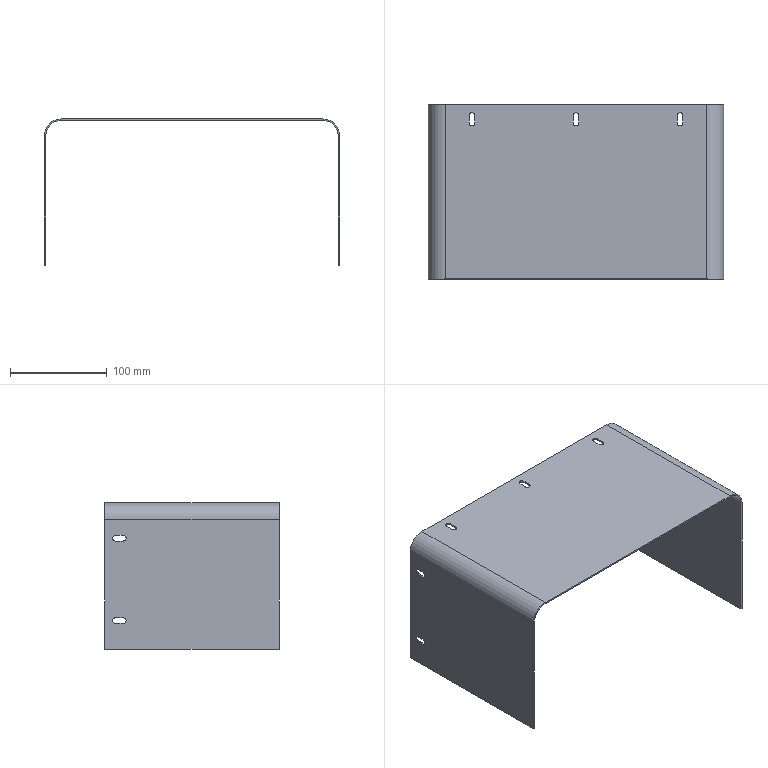Part | SolidWorks | features Fillet 2, HoleWzd 2, Shell 2, Extrusion 1, ICE 1 | 1 solid | 42 faces | box 305 x 180 x 151 mm | volume 158433 mm3 | plane 24 | cylinder 18 | commonest cylinder face diameters 5.8 x14 32 x2 35 x2
STEP:
#1=CARTESIAN_POINT('',(152.5,90.,58.));
#2=VERTEX_POINT('',#1);
#3=CARTESIAN_POINT('',(152.5,90.,-75.5));
#4=VERTEX_POINT('',#3);
#5=CARTESIAN_POINT('',(152.5,90.,75.5));
#6=DIRECTION('',(0.,0.,-1.));
#7=VECTOR('',#6,1000.);
#8=LINE('',#5,#7);
#9=EDGE_CURVE('',#2,#4,#8,.T.);
#10=ORIENTED_EDGE('',*,*,#9,.F.);
#11=CARTESIAN_POINT('',(152.5,-90.,58.));
#12=VERTEX_POINT('',#11);
#13=CARTESIAN_POINT('',(152.5,90.,58.));
#14=DIRECTION('',(0.,-1.,0.));
#15=VECTOR('',#14,1000.);
#16=LINE('',#13,#15);
#17=EDGE_CURVE('',#2,#12,#16,.T.);
#18=ORIENTED_EDGE('',*,*,#17,.T.);
#19=CARTESIAN_POINT('',(152.5,-90.,-75.5));
#20=VERTEX_POINT('',#19);
#21=CARTESIAN_POINT('',(152.5,-90.,75.5));
#22=DIRECTION('',(0.,0.,-1.));
#23=VECTOR('',#22,1000.);
#24=LINE('',#21,#23);
#25=EDGE_CURVE('',#12,#20,#24,.T.);
#26=ORIENTED_EDGE('',*,*,#25,.T.);
#27=CARTESIAN_POINT('',(152.5,90.,-75.5));
#28=DIRECTION('',(0.,-1.,0.));
#29=VECTOR('',#28,1000.);
#30=LINE('',#27,#29);
#31=EDGE_CURVE('',#4,#20,#30,.T.);
#32=ORIENTED_EDGE('',*,*,#31,.F.);
#33=EDGE_LOOP('',(#10,#18,#26,#32));
#34=FACE_OUTER_BOUND('',#33,.T.);
#35=CARTESIAN_POINT('',(152.5,71.,41.9));
#36=VERTEX_POINT('',#35);
#37=CARTESIAN_POINT('',(152.5,79.,41.9));
#38=VERTEX_POINT('',#37);
#39=CARTESIAN_POINT('',(152.5,71.,41.9));
#40=DIRECTION('',(0.,1.,0.));
#41=VECTOR('',#40,1000.);
#42=LINE('',#39,#41);
#43=EDGE_CURVE('',#36,#38,#42,.T.);
#44=ORIENTED_EDGE('',*,*,#43,.T.);
#45=CARTESIAN_POINT('',(152.5,79.,36.1));
#46=VERTEX_POINT('',#45);
#47=CARTESIAN_POINT('',(152.5,79.,39.));
#48=DIRECTION('',(-1.,0.,0.));
#49=DIRECTION('',(0.,0.,1.));
#50=AXIS2_PLACEMENT_3D('',#47,#48,#49);
#51=CIRCLE('',#50,2.9);
#52=EDGE_CURVE('',#38,#46,#51,.T.);
#53=ORIENTED_EDGE('',*,*,#52,.T.);
#54=CARTESIAN_POINT('',(152.5,71.,36.1));
#55=VERTEX_POINT('',#54);
#56=CARTESIAN_POINT('',(152.5,71.,36.1));
#57=DIRECTION('',(0.,1.,0.));
#58=VECTOR('',#57,1000.);
#59=LINE('',#56,#58);
#60=EDGE_CURVE('',#55,#46,#59,.T.);
#61=ORIENTED_EDGE('',*,*,#60,.F.);
#62=CARTESIAN_POINT('',(152.5,71.,39.));
#63=DIRECTION('',(-1.,0.,0.));
#64=DIRECTION('',(0.,0.,1.));
#65=AXIS2_PLACEMENT_3D('',#62,#63,#64);
#66=CIRCLE('',#65,2.9);
#67=EDGE_CURVE('',#55,#36,#66,.T.);
#68=ORIENTED_EDGE('',*,*,#67,.T.);
#69=EDGE_LOOP('',(#44,#53,#61,#68));
#70=FACE_BOUND('',#69,.T.);
#71=CARTESIAN_POINT('',(152.5,71.,-48.9));
#72=VERTEX_POINT('',#71);
#73=CARTESIAN_POINT('',(152.5,79.,-48.9));
#74=VERTEX_POINT('',#73);
#75=CARTESIAN_POINT('',(152.5,71.,-48.9));
#76=DIRECTION('',(0.,1.,0.));
#77=VECTOR('',#76,1000.);
#78=LINE('',#75,#77);
#79=EDGE_CURVE('',#72,#74,#78,.T.);
#80=ORIENTED_EDGE('',*,*,#79,.F.);
#81=CARTESIAN_POINT('',(152.5,71.,-43.1));
#82=VERTEX_POINT('',#81);
#83=CARTESIAN_POINT('',(152.5,71.,-46.));
#84=DIRECTION('',(-1.,0.,0.));
#85=DIRECTION('',(0.,0.,1.));
#86=AXIS2_PLACEMENT_3D('',#83,#84,#85);
#87=CIRCLE('',#86,2.9);
#88=EDGE_CURVE('',#72,#82,#87,.T.);
#89=ORIENTED_EDGE('',*,*,#88,.T.);
#90=CARTESIAN_POINT('',(152.5,79.,-43.1));
#91=VERTEX_POINT('',#90);
#92=CARTESIAN_POINT('',(152.5,71.,-43.1));
#93=DIRECTION('',(0.,1.,0.));
#94=VECTOR('',#93,1000.);
#95=LINE('',#92,#94);
#96=EDGE_CURVE('',#82,#91,#95,.T.);
#97=ORIENTED_EDGE('',*,*,#96,.T.);
#98=CARTESIAN_POINT('',(152.5,79.,-46.));
#99=DIRECTION('',(-1.,0.,0.));
#100=DIRECTION('',(0.,0.,1.));
#101=AXIS2_PLACEMENT_3D('',#98,#99,#100);
#102=CIRCLE('',#101,2.9);
#103=EDGE_CURVE('',#91,#74,#102,.T.);
#104=ORIENTED_EDGE('',*,*,#103,.T.);
#105=EDGE_LOOP('',(#80,#89,#97,#104));
#106=FACE_BOUND('',#105,.T.);
#107=CARTESIAN_POINT('',(152.5,90.,75.5));
#108=DIRECTION('',(-1.,0.,0.));
#109=DIRECTION('',(0.,0.,1.));
#110=AXIS2_PLACEMENT_3D('',#107,#108,#109);
#111=PLANE('',#110);
#112=ADVANCED_FACE('',(#34,#70,#106),#111,.F.);
#113=CARTESIAN_POINT('',(151.,90.,-75.5));
#114=VERTEX_POINT('',#113);
#115=CARTESIAN_POINT('',(151.,-90.,-75.5));
#116=VERTEX_POINT('',#115);
#117=CARTESIAN_POINT('',(151.,90.,-75.5));
#118=DIRECTION('',(0.,-1.,0.));
#119=VECTOR('',#118,1000.);
#120=LINE('',#117,#119);
#121=EDGE_CURVE('',#114,#116,#120,.T.);
#122=ORIENTED_EDGE('',*,*,#121,.F.);
#123=CARTESIAN_POINT('',(-152.5,90.,-75.5));
#124=DIRECTION('',(-1.,0.,0.));
#125=VECTOR('',#124,1000.);
#126=LINE('',#123,#125);
#127=EDGE_CURVE('',#4,#114,#126,.T.);
#128=ORIENTED_EDGE('',*,*,#127,.F.);
#129=ORIENTED_EDGE('',*,*,#31,.T.);
#130=CARTESIAN_POINT('',(-152.5,-90.,-75.5));
#131=DIRECTION('',(-1.,0.,0.));
#132=VECTOR('',#131,1000.);
#133=LINE('',#130,#132);
#134=EDGE_CURVE('',#20,#116,#133,.T.);
#135=ORIENTED_EDGE('',*,*,#134,.T.);
#136=EDGE_LOOP('',(#122,#128,#129,#135));
#137=FACE_OUTER_BOUND('',#136,.T.);
#138=CARTESIAN_POINT('',(-152.5,90.,-75.5));
#139=DIRECTION('',(0.,0.,1.));
#140=DIRECTION('',(1.,0.,0.));
#141=AXIS2_PLACEMENT_3D('',#138,#139,#140);
#142=PLANE('',#141);
#143=ADVANCED_FACE('',(#137),#142,.F.);
#144=CARTESIAN_POINT('',(151.,-90.,58.));
#145=VERTEX_POINT('',#144);
#146=CARTESIAN_POINT('',(135.,-90.,74.));
#147=VERTEX_POINT('',#146);
#148=CARTESIAN_POINT('',(135.,-90.,58.));
#149=DIRECTION('',(0.,-1.,0.));
#150=DIRECTION('',(0.,0.,-1.));
#151=AXIS2_PLACEMENT_3D('',#148,#149,#150);
#152=CIRCLE('',#151,16.);
#153=EDGE_CURVE('',#145,#147,#152,.T.);
#154=ORIENTED_EDGE('',*,*,#153,.F.);
#155=CARTESIAN_POINT('',(151.,-90.,0.));
#156=DIRECTION('',(0.,0.,-1.));
#157=VECTOR('',#156,1000.);
#158=LINE('',#155,#157);
#159=EDGE_CURVE('',#145,#116,#158,.T.);
#160=ORIENTED_EDGE('',*,*,#159,.T.);
#161=ORIENTED_EDGE('',*,*,#134,.F.);
#162=ORIENTED_EDGE('',*,*,#25,.F.);
#163=CARTESIAN_POINT('',(135.,-90.,75.5));
#164=VERTEX_POINT('',#163);
#165=CARTESIAN_POINT('',(135.,-90.,58.));
#166=DIRECTION('',(0.,-1.,0.));
#167=DIRECTION('',(0.,0.,-1.));
#168=AXIS2_PLACEMENT_3D('',#165,#166,#167);
#169=CIRCLE('',#168,17.5);
#170=EDGE_CURVE('',#12,#164,#169,.T.);
#171=ORIENTED_EDGE('',*,*,#170,.T.);
#172=CARTESIAN_POINT('',(-135.,-90.,75.5));
#173=VERTEX_POINT('',#172);
#174=CARTESIAN_POINT('',(-152.5,-90.,75.5));
#175=DIRECTION('',(1.,0.,0.));
#176=VECTOR('',#175,1000.);
#177=LINE('',#174,#176);
#178=EDGE_CURVE('',#173,#164,#177,.T.);
#179=ORIENTED_EDGE('',*,*,#178,.F.);
#180=CARTESIAN_POINT('',(-152.5,-90.,58.));
#181=VERTEX_POINT('',#180);
#182=CARTESIAN_POINT('',(-135.,-90.,58.));
#183=DIRECTION('',(0.,-1.,0.));
#184=DIRECTION('',(0.,0.,-1.));
#185=AXIS2_PLACEMENT_3D('',#182,#183,#184);
#186=CIRCLE('',#185,17.5);
#187=EDGE_CURVE('',#173,#181,#186,.T.);
#188=ORIENTED_EDGE('',*,*,#187,.T.);
#189=CARTESIAN_POINT('',(-152.5,-90.,-75.5));
#190=VERTEX_POINT('',#189);
#191=CARTESIAN_POINT('',(-152.5,-90.,75.5));
#192=DIRECTION('',(0.,0.,1.));
#193=VECTOR('',#192,1000.);
#194=LINE('',#191,#193);
#195=EDGE_CURVE('',#190,#181,#194,.T.);
#196=ORIENTED_EDGE('',*,*,#195,.F.);
#197=CARTESIAN_POINT('',(-151.,-90.,-75.5));
#198=VERTEX_POINT('',#197);
#199=CARTESIAN_POINT('',(-152.5,-90.,-75.5));
#200=DIRECTION('',(-1.,0.,0.));
#201=VECTOR('',#200,1000.);
#202=LINE('',#199,#201);
#203=EDGE_CURVE('',#198,#190,#202,.T.);
#204=ORIENTED_EDGE('',*,*,#203,.F.);
#205=CARTESIAN_POINT('',(-151.,-90.,58.));
#206=VERTEX_POINT('',#205);
#207=CARTESIAN_POINT('',(-151.,-90.,0.));
#208=DIRECTION('',(0.,0.,1.));
#209=VECTOR('',#208,1000.);
#210=LINE('',#207,#209);
#211=EDGE_CURVE('',#198,#206,#210,.T.);
#212=ORIENTED_EDGE('',*,*,#211,.T.);
#213=CARTESIAN_POINT('',(-135.,-90.,74.));
#214=VERTEX_POINT('',#213);
#215=CARTESIAN_POINT('',(-135.,-90.,58.));
#216=DIRECTION('',(0.,-1.,0.));
#217=DIRECTION('',(0.,0.,-1.));
#218=AXIS2_PLACEMENT_3D('',#215,#216,#217);
#219=CIRCLE('',#218,16.);
#220=EDGE_CURVE('',#214,#206,#219,.T.);
#221=ORIENTED_EDGE('',*,*,#220,.F.);
#222=CARTESIAN_POINT('',(0.,-90.,74.));
#223=DIRECTION('',(1.,0.,0.));
#224=VECTOR('',#223,1000.);
#225=LINE('',#222,#224);
#226=EDGE_CURVE('',#214,#147,#225,.T.);
#227=ORIENTED_EDGE('',*,*,#226,.T.);
#228=EDGE_LOOP('',(#154,#160,#161,#162,#171,#179,#188,#196,#204,#212,#221,#227));
#229=FACE_OUTER_BOUND('',#228,.T.);
#230=CARTESIAN_POINT('',(0.,-90.,0.));
#231=DIRECTION('',(0.,-1.,0.));
#232=DIRECTION('',(0.,0.,-1.));
#233=AXIS2_PLACEMENT_3D('',#230,#231,#232);
#234=PLANE('',#233);
#235=ADVANCED_FACE('',(#229),#234,.T.);
#236=CARTESIAN_POINT('',(-151.,90.,-75.5));
#237=VERTEX_POINT('',#236);
#238=CARTESIAN_POINT('',(-152.5,90.,-75.5));
#239=VERTEX_POINT('',#238);
#240=CARTESIAN_POINT('',(-152.5,90.,-75.5));
#241=DIRECTION('',(-1.,0.,0.));
#242=VECTOR('',#241,1000.);
#243=LINE('',#240,#242);
#244=EDGE_CURVE('',#237,#239,#243,.T.);
#245=ORIENTED_EDGE('',*,*,#244,.F.);
#246=CARTESIAN_POINT('',(-151.,90.,-75.5));
#247=DIRECTION('',(0.,-1.,0.));
#248=VECTOR('',#247,1000.);
#249=LINE('',#246,#248);
#250=EDGE_CURVE('',#237,#198,#249,.T.);
#251=ORIENTED_EDGE('',*,*,#250,.T.);
#252=ORIENTED_EDGE('',*,*,#203,.T.);
#253=CARTESIAN_POINT('',(-152.5,90.,-75.5));
#254=DIRECTION('',(0.,-1.,0.));
#255=VECTOR('',#254,1000.);
#256=LINE('',#253,#255);
#257=EDGE_CURVE('',#239,#190,#256,.T.);
#258=ORIENTED_EDGE('',*,*,#257,.F.);
#259=EDGE_LOOP('',(#245,#251,#252,#258));
#260=FACE_OUTER_BOUND('',#259,.T.);
#261=CARTESIAN_POINT('',(-152.5,90.,-75.5));
#262=DIRECTION('',(0.,0.,1.));
#263=DIRECTION('',(1.,0.,0.));
#264=AXIS2_PLACEMENT_3D('',#261,#262,#263);
#265=PLANE('',#264);
#266=ADVANCED_FACE('',(#260),#265,.F.);
#267=CARTESIAN_POINT('',(-152.5,71.,-48.9));
#268=VERTEX_POINT('',#267);
#269=CARTESIAN_POINT('',(-152.5,71.,-43.1));
#270=VERTEX_POINT('',#269);
#271=CARTESIAN_POINT('',(-152.5,71.,-46.));
#272=DIRECTION('',(-1.,0.,0.));
#273=DIRECTION('',(0.,0.,1.));
#274=AXIS2_PLACEMENT_3D('',#271,#272,#273);
#275=CIRCLE('',#274,2.9);
#276=EDGE_CURVE('',#268,#270,#275,.T.);
#277=ORIENTED_EDGE('',*,*,#276,.F.);
#278=CARTESIAN_POINT('',(-152.5,79.,-48.9));
#279=VERTEX_POINT('',#278);
#280=CARTESIAN_POINT('',(-152.5,71.,-48.9));
#281=DIRECTION('',(0.,1.,0.));
#282=VECTOR('',#281,1000.);
#283=LINE('',#280,#282);
#284=EDGE_CURVE('',#268,#279,#283,.T.);
#285=ORIENTED_EDGE('',*,*,#284,.T.);
#286=CARTESIAN_POINT('',(-152.5,79.,-43.1));
#287=VERTEX_POINT('',#286);
#288=CARTESIAN_POINT('',(-152.5,79.,-46.));
#289=DIRECTION('',(-1.,0.,0.));
#290=DIRECTION('',(0.,0.,1.));
#291=AXIS2_PLACEMENT_3D('',#288,#289,#290);
#292=CIRCLE('',#291,2.9);
#293=EDGE_CURVE('',#287,#279,#292,.T.);
#294=ORIENTED_EDGE('',*,*,#293,.F.);
#295=CARTESIAN_POINT('',(-152.5,71.,-43.1));
#296=DIRECTION('',(0.,1.,0.));
#297=VECTOR('',#296,1000.);
#298=LINE('',#295,#297);
#299=EDGE_CURVE('',#270,#287,#298,.T.);
#300=ORIENTED_EDGE('',*,*,#299,.F.);
#301=EDGE_LOOP('',(#277,#285,#294,#300));
#302=FACE_BOUND('',#301,.T.);
#303=CARTESIAN_POINT('',(-152.5,71.,36.1));
#304=VERTEX_POINT('',#303);
#305=CARTESIAN_POINT('',(-152.5,71.,41.9));
#306=VERTEX_POINT('',#305);
#307=CARTESIAN_POINT('',(-152.5,71.,39.));
#308=DIRECTION('',(-1.,0.,0.));
#309=DIRECTION('',(0.,0.,1.));
#310=AXIS2_PLACEMENT_3D('',#307,#308,#309);
#311=CIRCLE('',#310,2.9);
#312=EDGE_CURVE('',#304,#306,#311,.T.);
#313=ORIENTED_EDGE('',*,*,#312,.F.);
#314=CARTESIAN_POINT('',(-152.5,79.,36.1));
#315=VERTEX_POINT('',#314);
#316=CARTESIAN_POINT('',(-152.5,71.,36.1));
#317=DIRECTION('',(0.,1.,0.));
#318=VECTOR('',#317,1000.);
#319=LINE('',#316,#318);
#320=EDGE_CURVE('',#304,#315,#319,.T.);
#321=ORIENTED_EDGE('',*,*,#320,.T.);
#322=CARTESIAN_POINT('',(-152.5,79.,41.9));
#323=VERTEX_POINT('',#322);
#324=CARTESIAN_POINT('',(-152.5,79.,39.));
#325=DIRECTION('',(-1.,0.,0.));
#326=DIRECTION('',(0.,0.,1.));
#327=AXIS2_PLACEMENT_3D('',#324,#325,#326);
#328=CIRCLE('',#327,2.9);
#329=EDGE_CURVE('',#323,#315,#328,.T.);
#330=ORIENTED_EDGE('',*,*,#329,.F.);
#331=CARTESIAN_POINT('',(-152.5,71.,41.9));
#332=DIRECTION('',(0.,1.,0.));
#333=VECTOR('',#332,1000.);
#334=LINE('',#331,#333);
#335=EDGE_CURVE('',#306,#323,#334,.T.);
#336=ORIENTED_EDGE('',*,*,#335,.F.);
#337=EDGE_LOOP('',(#313,#321,#330,#336));
#338=FACE_BOUND('',#337,.T.);
#339=ORIENTED_EDGE('',*,*,#195,.T.);
#340=CARTESIAN_POINT('',(-152.5,90.,58.));
#341=VERTEX_POINT('',#340);
#342=CARTESIAN_POINT('',(-152.5,90.,58.));
#343=DIRECTION('',(0.,1.,0.));
#344=VECTOR('',#343,1000.);
#345=LINE('',#342,#344);
#346=EDGE_CURVE('',#181,#341,#345,.T.);
#347=ORIENTED_EDGE('',*,*,#346,.T.);
#348=CARTESIAN_POINT('',(-152.5,90.,75.5));
#349=DIRECTION('',(0.,0.,1.));
#350=VECTOR('',#349,1000.);
#351=LINE('',#348,#350);
#352=EDGE_CURVE('',#239,#341,#351,.T.);
#353=ORIENTED_EDGE('',*,*,#352,.F.);
#354=ORIENTED_EDGE('',*,*,#257,.T.);
#355=EDGE_LOOP('',(#339,#347,#353,#354));
#356=FACE_OUTER_BOUND('',#355,.T.);
#357=CARTESIAN_POINT('',(-152.5,90.,75.5));
#358=DIRECTION('',(1.,0.,0.));
#359=DIRECTION('',(0.,0.,-1.));
#360=AXIS2_PLACEMENT_3D('',#357,#358,#359);
#361=PLANE('',#360);
#362=ADVANCED_FACE('',(#302,#338,#356),#361,.F.);
#363=CARTESIAN_POINT('',(-110.4,71.,75.5));
#364=VERTEX_POINT('',#363);
#365=CARTESIAN_POINT('',(-104.6,71.,75.5));
#366=VERTEX_POINT('',#365);
#367=CARTESIAN_POINT('',(-107.5,71.,75.5));
#368=DIRECTION('',(0.,0.,1.));
#369=DIRECTION('',(1.,0.,0.));
#370=AXIS2_PLACEMENT_3D('',#367,#368,#369);
#371=CIRCLE('',#370,2.9);
#372=EDGE_CURVE('',#364,#366,#371,.T.);
#373=ORIENTED_EDGE('',*,*,#372,.F.);
#374=CARTESIAN_POINT('',(-110.4,79.,75.5));
#375=VERTEX_POINT('',#374);
#376=CARTESIAN_POINT('',(-110.4,71.,75.5));
#377=DIRECTION('',(0.,1.,0.));
#378=VECTOR('',#377,1000.);
#379=LINE('',#376,#378);
#380=EDGE_CURVE('',#364,#375,#379,.T.);
#381=ORIENTED_EDGE('',*,*,#380,.T.);
#382=CARTESIAN_POINT('',(-104.6,79.,75.5));
#383=VERTEX_POINT('',#382);
#384=CARTESIAN_POINT('',(-107.5,79.,75.5));
#385=DIRECTION('',(0.,0.,1.));
#386=DIRECTION('',(1.,0.,0.));
#387=AXIS2_PLACEMENT_3D('',#384,#385,#386);
#388=CIRCLE('',#387,2.9);
#389=EDGE_CURVE('',#383,#375,#388,.T.);
#390=ORIENTED_EDGE('',*,*,#389,.F.);
#391=CARTESIAN_POINT('',(-104.6,71.,75.5));
#392=DIRECTION('',(0.,1.,0.));
#393=VECTOR('',#392,1000.);
#394=LINE('',#391,#393);
#395=EDGE_CURVE('',#366,#383,#394,.T.);
#396=ORIENTED_EDGE('',*,*,#395,.F.);
#397=EDGE_LOOP('',(#373,#381,#390,#396));
#398=FACE_BOUND('',#397,.T.);
#399=CARTESIAN_POINT('',(-2.9,71.,75.5));
#400=VERTEX_POINT('',#399);
#401=CARTESIAN_POINT('',(2.9,71.,75.5));
#402=VERTEX_POINT('',#401);
#403=CARTESIAN_POINT('',(0.,71.,75.5));
#404=DIRECTION('',(0.,0.,1.));
#405=DIRECTION('',(1.,0.,0.));
#406=AXIS2_PLACEMENT_3D('',#403,#404,#405);
#407=CIRCLE('',#406,2.9);
#408=EDGE_CURVE('',#400,#402,#407,.T.);
#409=ORIENTED_EDGE('',*,*,#408,.F.);
#410=CARTESIAN_POINT('',(-2.9,79.,75.5));
#411=VERTEX_POINT('',#410);
#412=CARTESIAN_POINT('',(-2.9,71.,75.5));
#413=DIRECTION('',(0.,1.,0.));
#414=VECTOR('',#413,1000.);
#415=LINE('',#412,#414);
#416=EDGE_CURVE('',#400,#411,#415,.T.);
#417=ORIENTED_EDGE('',*,*,#416,.T.);
#418=CARTESIAN_POINT('',(2.9,79.,75.5));
#419=VERTEX_POINT('',#418);
#420=CARTESIAN_POINT('',(0.,79.,75.5));
#421=DIRECTION('',(0.,0.,1.));
#422=DIRECTION('',(1.,0.,0.));
#423=AXIS2_PLACEMENT_3D('',#420,#421,#422);
#424=CIRCLE('',#423,2.9);
#425=EDGE_CURVE('',#419,#411,#424,.T.);
#426=ORIENTED_EDGE('',*,*,#425,.F.);
#427=CARTESIAN_POINT('',(2.9,71.,75.5));
#428=DIRECTION('',(0.,1.,0.));
#429=VECTOR('',#428,1000.);
#430=LINE('',#427,#429);
#431=EDGE_CURVE('',#402,#419,#430,.T.);
#432=ORIENTED_EDGE('',*,*,#431,.F.);
#433=EDGE_LOOP('',(#409,#417,#426,#432));
#434=FACE_BOUND('',#433,.T.);
#435=CARTESIAN_POINT('',(104.6,71.,75.5));
#436=VERTEX_POINT('',#435);
#437=CARTESIAN_POINT('',(110.4,71.,75.5));
#438=VERTEX_POINT('',#437);
#439=CARTESIAN_POINT('',(107.5,71.,75.5));
#440=DIRECTION('',(0.,0.,1.));
#441=DIRECTION('',(1.,0.,0.));
#442=AXIS2_PLACEMENT_3D('',#439,#440,#441);
#443=CIRCLE('',#442,2.9);
#444=EDGE_CURVE('',#436,#438,#443,.T.);
#445=ORIENTED_EDGE('',*,*,#444,.F.);
#446=CARTESIAN_POINT('',(104.6,79.,75.5));
#447=VERTEX_POINT('',#446);
#448=CARTESIAN_POINT('',(104.6,71.,75.5));
#449=DIRECTION('',(0.,1.,0.));
#450=VECTOR('',#449,1000.);
#451=LINE('',#448,#450);
#452=EDGE_CURVE('',#436,#447,#451,.T.);
#453=ORIENTED_EDGE('',*,*,#452,.T.);
#454=CARTESIAN_POINT('',(110.4,79.,75.5));
#455=VERTEX_POINT('',#454);
#456=CARTESIAN_POINT('',(107.5,79.,75.5));
#457=DIRECTION('',(0.,0.,1.));
#458=DIRECTION('',(1.,0.,0.));
#459=AXIS2_PLACEMENT_3D('',#456,#457,#458);
#460=CIRCLE('',#459,2.9);
#461=EDGE_CURVE('',#455,#447,#460,.T.);
#462=ORIENTED_EDGE('',*,*,#461,.F.);
#463=CARTESIAN_POINT('',(110.4,71.,75.5));
#464=DIRECTION('',(0.,1.,0.));
#465=VECTOR('',#464,1000.);
#466=LINE('',#463,#465);
#467=EDGE_CURVE('',#438,#455,#466,.T.);
#468=ORIENTED_EDGE('',*,*,#467,.F.);
#469=EDGE_LOOP('',(#445,#453,#462,#468));
#470=FACE_BOUND('',#469,.T.);
#471=ORIENTED_EDGE('',*,*,#178,.T.);
#472=CARTESIAN_POINT('',(135.,90.,75.5));
#473=VERTEX_POINT('',#472);
#474=CARTESIAN_POINT('',(135.,90.,75.5));
#475=DIRECTION('',(0.,1.,0.));
#476=VECTOR('',#475,1000.);
#477=LINE('',#474,#476);
#478=EDGE_CURVE('',#164,#473,#477,.T.);
#479=ORIENTED_EDGE('',*,*,#478,.T.);
#480=CARTESIAN_POINT('',(-135.,90.,75.5));
#481=VERTEX_POINT('',#480);
#482=CARTESIAN_POINT('',(-152.5,90.,75.5));
#483=DIRECTION('',(1.,0.,0.));
#484=VECTOR('',#483,1000.);
#485=LINE('',#482,#484);
#486=EDGE_CURVE('',#481,#473,#485,.T.);
#487=ORIENTED_EDGE('',*,*,#486,.F.);
#488=CARTESIAN_POINT('',(-135.,90.,75.5));
#489=DIRECTION('',(0.,-1.,0.));
#490=VECTOR('',#489,1000.);
#491=LINE('',#488,#490);
#492=EDGE_CURVE('',#481,#173,#491,.T.);
#493=ORIENTED_EDGE('',*,*,#492,.T.);
#494=EDGE_LOOP('',(#471,#479,#487,#493));
#495=FACE_OUTER_BOUND('',#494,.T.);
#496=CARTESIAN_POINT('',(-152.5,90.,75.5));
#497=DIRECTION('',(0.,0.,-1.));
#498=DIRECTION('',(-1.,0.,0.));
#499=AXIS2_PLACEMENT_3D('',#496,#497,#498);
#500=PLANE('',#499);
#501=ADVANCED_FACE('',(#398,#434,#470,#495),#500,.F.);
#502=CARTESIAN_POINT('',(151.,90.,58.));
#503=VERTEX_POINT('',#502);
#504=CARTESIAN_POINT('',(151.,90.,0.));
#505=DIRECTION('',(0.,0.,-1.));
#506=VECTOR('',#505,1000.);
#507=LINE('',#504,#506);
#508=EDGE_CURVE('',#503,#114,#507,.T.);
#509=ORIENTED_EDGE('',*,*,#508,.F.);
#510=CARTESIAN_POINT('',(135.,90.,74.));
#511=VERTEX_POINT('',#510);
#512=CARTESIAN_POINT('',(135.,90.,58.));
#513=DIRECTION('',(0.,1.,0.));
#514=DIRECTION('',(0.,0.,-1.));
#515=AXIS2_PLACEMENT_3D('',#512,#513,#514);
#516=CIRCLE('',#515,16.);
#517=EDGE_CURVE('',#511,#503,#516,.T.);
#518=ORIENTED_EDGE('',*,*,#517,.F.);
#519=CARTESIAN_POINT('',(-135.,90.,74.));
#520=VERTEX_POINT('',#519);
#521=CARTESIAN_POINT('',(0.,90.,74.));
#522=DIRECTION('',(1.,0.,0.));
#523=VECTOR('',#522,1000.);
#524=LINE('',#521,#523);
#525=EDGE_CURVE('',#520,#511,#524,.T.);
#526=ORIENTED_EDGE('',*,*,#525,.F.);
#527=CARTESIAN_POINT('',(-151.,90.,58.));
#528=VERTEX_POINT('',#527);
#529=CARTESIAN_POINT('',(-135.,90.,58.));
#530=DIRECTION('',(0.,1.,0.));
#531=DIRECTION('',(0.,0.,-1.));
#532=AXIS2_PLACEMENT_3D('',#529,#530,#531);
#533=CIRCLE('',#532,16.);
#534=EDGE_CURVE('',#528,#520,#533,.T.);
#535=ORIENTED_EDGE('',*,*,#534,.F.);
#536=CARTESIAN_POINT('',(-151.,90.,0.));
#537=DIRECTION('',(0.,0.,1.));
#538=VECTOR('',#537,1000.);
#539=LINE('',#536,#538);
#540=EDGE_CURVE('',#237,#528,#539,.T.);
#541=ORIENTED_EDGE('',*,*,#540,.F.);
#542=ORIENTED_EDGE('',*,*,#244,.T.);
#543=ORIENTED_EDGE('',*,*,#352,.T.);
#544=CARTESIAN_POINT('',(-135.,90.,58.));
#545=DIRECTION('',(0.,1.,0.));
#546=DIRECTION('',(0.,0.,-1.));
#547=AXIS2_PLACEMENT_3D('',#544,#545,#546);
#548=CIRCLE('',#547,17.5);
#549=EDGE_CURVE('',#341,#481,#548,.T.);
#550=ORIENTED_EDGE('',*,*,#549,.T.);
#551=ORIENTED_EDGE('',*,*,#486,.T.);
#552=CARTESIAN_POINT('',(135.,90.,58.));
#553=DIRECTION('',(0.,1.,0.));
#554=DIRECTION('',(0.,0.,-1.));
#555=AXIS2_PLACEMENT_3D('',#552,#553,#554);
#556=CIRCLE('',#555,17.5);
#557=EDGE_CURVE('',#473,#2,#556,.T.);
#558=ORIENTED_EDGE('',*,*,#557,.T.);
#559=ORIENTED_EDGE('',*,*,#9,.T.);
#560=ORIENTED_EDGE('',*,*,#127,.T.);
#561=EDGE_LOOP('',(#509,#518,#526,#535,#541,#542,#543,#550,#551,#558,#559,#560));
#562=FACE_OUTER_BOUND('',#561,.T.);
#563=CARTESIAN_POINT('',(0.,90.,0.));
#564=DIRECTION('',(0.,-1.,0.));
#565=DIRECTION('',(0.,0.,-1.));
#566=AXIS2_PLACEMENT_3D('',#563,#564,#565);
#567=PLANE('',#566);
#568=ADVANCED_FACE('',(#562),#567,.F.);
#569=ORIENTED_EDGE('',*,*,#557,.F.);
#570=ORIENTED_EDGE('',*,*,#478,.F.);
#571=ORIENTED_EDGE('',*,*,#170,.F.);
#572=ORIENTED_EDGE('',*,*,#17,.F.);
#573=EDGE_LOOP('',(#569,#570,#571,#572));
#574=FACE_OUTER_BOUND('',#573,.T.);
#575=CARTESIAN_POINT('',(135.,90.,58.));
#576=DIRECTION('',(0.,-1.,0.));
#577=DIRECTION('',(0.,0.,-1.));
#578=AXIS2_PLACEMENT_3D('',#575,#576,#577);
#579=CYLINDRICAL_SURFACE('',#578,17.5);
#580=ADVANCED_FACE('',(#574),#579,.T.);
#581=ORIENTED_EDGE('',*,*,#549,.F.);
#582=ORIENTED_EDGE('',*,*,#346,.F.);
#583=ORIENTED_EDGE('',*,*,#187,.F.);
#584=ORIENTED_EDGE('',*,*,#492,.F.);
#585=EDGE_LOOP('',(#581,#582,#583,#584));
#586=FACE_OUTER_BOUND('',#585,.T.);
#587=CARTESIAN_POINT('',(-135.,90.,58.));
#588=DIRECTION('',(0.,-1.,0.));
#589=DIRECTION('',(0.,0.,-1.));
#590=AXIS2_PLACEMENT_3D('',#587,#588,#589);
#591=CYLINDRICAL_SURFACE('',#590,17.5);
#592=ADVANCED_FACE('',(#586),#591,.T.);
#593=CARTESIAN_POINT('',(151.,71.,-43.1));
#594=VERTEX_POINT('',#593);
#595=CARTESIAN_POINT('',(151.,79.,-43.1));
#596=VERTEX_POINT('',#595);
#597=CARTESIAN_POINT('',(151.,90.,-43.1));
#598=DIRECTION('',(0.,1.,0.));
#599=VECTOR('',#598,1000.);
#600=LINE('',#597,#599);
#601=EDGE_CURVE('',#594,#596,#600,.T.);
#602=ORIENTED_EDGE('',*,*,#601,.F.);
#603=CARTESIAN_POINT('',(151.,71.,-48.9));
#604=VERTEX_POINT('',#603);
#605=CARTESIAN_POINT('',(151.,71.,-46.));
#606=DIRECTION('',(-1.,0.,0.));
#607=DIRECTION('',(0.,0.,1.));
#608=AXIS2_PLACEMENT_3D('',#605,#606,#607);
#609=CIRCLE('',#608,2.9);
#610=EDGE_CURVE('',#604,#594,#609,.T.);
#611=ORIENTED_EDGE('',*,*,#610,.F.);
#612=CARTESIAN_POINT('',(151.,79.,-48.9));
#613=VERTEX_POINT('',#612);
#614=CARTESIAN_POINT('',(151.,90.,-48.9));
#615=DIRECTION('',(0.,-1.,0.));
#616=VECTOR('',#615,1000.);
#617=LINE('',#614,#616);
#618=EDGE_CURVE('',#613,#604,#617,.T.);
#619=ORIENTED_EDGE('',*,*,#618,.F.);
#620=CARTESIAN_POINT('',(151.,79.,-46.));
#621=DIRECTION('',(-1.,0.,0.));
#622=DIRECTION('',(0.,0.,1.));
#623=AXIS2_PLACEMENT_3D('',#620,#621,#622);
#624=CIRCLE('',#623,2.9);
#625=EDGE_CURVE('',#596,#613,#624,.T.);
#626=ORIENTED_EDGE('',*,*,#625,.F.);
#627=EDGE_LOOP('',(#602,#611,#619,#626));
#628=FACE_BOUND('',#627,.T.);
#629=CARTESIAN_POINT('',(151.,79.,36.1));
#630=VERTEX_POINT('',#629);
#631=CARTESIAN_POINT('',(151.,71.,36.1));
#632=VERTEX_POINT('',#631);
#633=CARTESIAN_POINT('',(151.,90.,36.1));
#634=DIRECTION('',(0.,-1.,0.));
#635=VECTOR('',#634,1000.);
#636=LINE('',#633,#635);
#637=EDGE_CURVE('',#630,#632,#636,.T.);
#638=ORIENTED_EDGE('',*,*,#637,.F.);
#639=CARTESIAN_POINT('',(151.,79.,41.9));
#640=VERTEX_POINT('',#639);
#641=CARTESIAN_POINT('',(151.,79.,39.));
#642=DIRECTION('',(-1.,0.,0.));
#643=DIRECTION('',(0.,0.,1.));
#644=AXIS2_PLACEMENT_3D('',#641,#642,#643);
#645=CIRCLE('',#644,2.9);
#646=EDGE_CURVE('',#640,#630,#645,.T.);
#647=ORIENTED_EDGE('',*,*,#646,.F.);
#648=CARTESIAN_POINT('',(151.,71.,41.9));
#649=VERTEX_POINT('',#648);
#650=CARTESIAN_POINT('',(151.,90.,41.9));
#651=DIRECTION('',(0.,1.,0.));
#652=VECTOR('',#651,1000.);
#653=LINE('',#650,#652);
#654=EDGE_CURVE('',#649,#640,#653,.T.);
#655=ORIENTED_EDGE('',*,*,#654,.F.);
#656=CARTESIAN_POINT('',(151.,71.,39.));
#657=DIRECTION('',(-1.,0.,0.));
#658=DIRECTION('',(0.,0.,1.));
#659=AXIS2_PLACEMENT_3D('',#656,#657,#658);
#660=CIRCLE('',#659,2.9);
#661=EDGE_CURVE('',#632,#649,#660,.T.);
#662=ORIENTED_EDGE('',*,*,#661,.F.);
#663=EDGE_LOOP('',(#638,#647,#655,#662));
#664=FACE_BOUND('',#663,.T.);
#665=ORIENTED_EDGE('',*,*,#508,.T.);
#666=ORIENTED_EDGE('',*,*,#121,.T.);
#667=ORIENTED_EDGE('',*,*,#159,.F.);
#668=CARTESIAN_POINT('',(151.,90.,58.));
#669=DIRECTION('',(0.,-1.,0.));
#670=VECTOR('',#669,1000.);
#671=LINE('',#668,#670);
#672=EDGE_CURVE('',#503,#145,#671,.T.);
#673=ORIENTED_EDGE('',*,*,#672,.F.);
#674=EDGE_LOOP('',(#665,#666,#667,#673));
#675=FACE_OUTER_BOUND('',#674,.T.);
#676=CARTESIAN_POINT('',(151.,90.,75.5));
#677=DIRECTION('',(-1.,0.,0.));
#678=DIRECTION('',(0.,0.,1.));
#679=AXIS2_PLACEMENT_3D('',#676,#677,#678);
#680=PLANE('',#679);
#681=ADVANCED_FACE('',(#628,#664,#675),#680,.T.);
#682=CARTESIAN_POINT('',(-151.,71.,-48.9));
#683=VERTEX_POINT('',#682);
#684=CARTESIAN_POINT('',(-151.,79.,-48.9));
#685=VERTEX_POINT('',#684);
#686=CARTESIAN_POINT('',(-151.,90.,-48.9));
#687=DIRECTION('',(0.,1.,0.));
#688=VECTOR('',#687,1000.);
#689=LINE('',#686,#688);
#690=EDGE_CURVE('',#683,#685,#689,.T.);
#691=ORIENTED_EDGE('',*,*,#690,.F.);
#692=CARTESIAN_POINT('',(-151.,71.,-43.1));
#693=VERTEX_POINT('',#692);
#694=CARTESIAN_POINT('',(-151.,71.,-46.));
#695=DIRECTION('',(1.,0.,0.));
#696=DIRECTION('',(0.,0.,-1.));
#697=AXIS2_PLACEMENT_3D('',#694,#695,#696);
#698=CIRCLE('',#697,2.9);
#699=EDGE_CURVE('',#693,#683,#698,.T.);
#700=ORIENTED_EDGE('',*,*,#699,.F.);
#701=CARTESIAN_POINT('',(-151.,79.,-43.1));
#702=VERTEX_POINT('',#701);
#703=CARTESIAN_POINT('',(-151.,90.,-43.1));
#704=DIRECTION('',(0.,-1.,0.));
#705=VECTOR('',#704,1000.);
#706=LINE('',#703,#705);
#707=EDGE_CURVE('',#702,#693,#706,.T.);
#708=ORIENTED_EDGE('',*,*,#707,.F.);
#709=CARTESIAN_POINT('',(-151.,79.,-46.));
#710=DIRECTION('',(1.,0.,0.));
#711=DIRECTION('',(0.,0.,-1.));
#712=AXIS2_PLACEMENT_3D('',#709,#710,#711);
#713=CIRCLE('',#712,2.9);
#714=EDGE_CURVE('',#685,#702,#713,.T.);
#715=ORIENTED_EDGE('',*,*,#714,.F.);
#716=EDGE_LOOP('',(#691,#700,#708,#715));
#717=FACE_BOUND('',#716,.T.);
#718=CARTESIAN_POINT('',(-151.,71.,36.1));
#719=VERTEX_POINT('',#718);
#720=CARTESIAN_POINT('',(-151.,79.,36.1));
#721=VERTEX_POINT('',#720);
#722=CARTESIAN_POINT('',(-151.,90.,36.1));
#723=DIRECTION('',(0.,1.,0.));
#724=VECTOR('',#723,1000.);
#725=LINE('',#722,#724);
#726=EDGE_CURVE('',#719,#721,#725,.T.);
#727=ORIENTED_EDGE('',*,*,#726,.F.);
#728=CARTESIAN_POINT('',(-151.,71.,41.9));
#729=VERTEX_POINT('',#728);
#730=CARTESIAN_POINT('',(-151.,71.,39.));
#731=DIRECTION('',(1.,0.,0.));
#732=DIRECTION('',(0.,0.,-1.));
#733=AXIS2_PLACEMENT_3D('',#730,#731,#732);
#734=CIRCLE('',#733,2.9);
#735=EDGE_CURVE('',#729,#719,#734,.T.);
#736=ORIENTED_EDGE('',*,*,#735,.F.);
#737=CARTESIAN_POINT('',(-151.,79.,41.9));
#738=VERTEX_POINT('',#737);
#739=CARTESIAN_POINT('',(-151.,90.,41.9));
#740=DIRECTION('',(0.,-1.,0.));
#741=VECTOR('',#740,1000.);
#742=LINE('',#739,#741);
#743=EDGE_CURVE('',#738,#729,#742,.T.);
#744=ORIENTED_EDGE('',*,*,#743,.F.);
#745=CARTESIAN_POINT('',(-151.,79.,39.));
#746=DIRECTION('',(1.,0.,0.));
#747=DIRECTION('',(0.,0.,-1.));
#748=AXIS2_PLACEMENT_3D('',#745,#746,#747);
#749=CIRCLE('',#748,2.9);
#750=EDGE_CURVE('',#721,#738,#749,.T.);
#751=ORIENTED_EDGE('',*,*,#750,.F.);
#752=EDGE_LOOP('',(#727,#736,#744,#751));
#753=FACE_BOUND('',#752,.T.);
#754=ORIENTED_EDGE('',*,*,#211,.F.);
#755=ORIENTED_EDGE('',*,*,#250,.F.);
#756=ORIENTED_EDGE('',*,*,#540,.T.);
#757=CARTESIAN_POINT('',(-151.,90.,58.));
#758=DIRECTION('',(0.,1.,0.));
#759=VECTOR('',#758,1000.);
#760=LINE('',#757,#759);
#761=EDGE_CURVE('',#206,#528,#760,.T.);
#762=ORIENTED_EDGE('',*,*,#761,.F.);
#763=EDGE_LOOP('',(#754,#755,#756,#762));
#764=FACE_OUTER_BOUND('',#763,.T.);
#765=CARTESIAN_POINT('',(-151.,90.,75.5));
#766=DIRECTION('',(1.,0.,0.));
#767=DIRECTION('',(0.,0.,-1.));
#768=AXIS2_PLACEMENT_3D('',#765,#766,#767);
#769=PLANE('',#768);
#770=ADVANCED_FACE('',(#717,#753,#764),#769,.T.);
#771=CARTESIAN_POINT('',(-110.4,79.,74.));
#772=VERTEX_POINT('',#771);
#773=CARTESIAN_POINT('',(-104.6,79.,74.));
#774=VERTEX_POINT('',#773);
#775=CARTESIAN_POINT('',(-107.5,79.,74.));
#776=DIRECTION('',(0.,0.,-1.));
#777=DIRECTION('',(-1.,0.,0.));
#778=AXIS2_PLACEMENT_3D('',#775,#776,#777);
#779=CIRCLE('',#778,2.9);
#780=EDGE_CURVE('',#772,#774,#779,.T.);
#781=ORIENTED_EDGE('',*,*,#780,.F.);
#782=CARTESIAN_POINT('',(-110.4,71.,74.));
#783=VERTEX_POINT('',#782);
#784=CARTESIAN_POINT('',(-110.4,90.,74.));
#785=DIRECTION('',(0.,1.,0.));
#786=VECTOR('',#785,1000.);
#787=LINE('',#784,#786);
#788=EDGE_CURVE('',#783,#772,#787,.T.);
#789=ORIENTED_EDGE('',*,*,#788,.F.);
#790=CARTESIAN_POINT('',(-104.6,71.,74.));
#791=VERTEX_POINT('',#790);
#792=CARTESIAN_POINT('',(-107.5,71.,74.));
#793=DIRECTION('',(0.,0.,-1.));
#794=DIRECTION('',(-1.,0.,0.));
#795=AXIS2_PLACEMENT_3D('',#792,#793,#794);
#796=CIRCLE('',#795,2.9);
#797=EDGE_CURVE('',#791,#783,#796,.T.);
#798=ORIENTED_EDGE('',*,*,#797,.F.);
#799=CARTESIAN_POINT('',(-104.6,90.,74.));
#800=DIRECTION('',(0.,-1.,0.));
#801=VECTOR('',#800,1000.);
#802=LINE('',#799,#801);
#803=EDGE_CURVE('',#774,#791,#802,.T.);
#804=ORIENTED_EDGE('',*,*,#803,.F.);
#805=EDGE_LOOP('',(#781,#789,#798,#804));
#806=FACE_BOUND('',#805,.T.);
#807=CARTESIAN_POINT('',(2.9,71.,74.));
#808=VERTEX_POINT('',#807);
#809=CARTESIAN_POINT('',(-2.9,71.,74.));
#810=VERTEX_POINT('',#809);
#811=CARTESIAN_POINT('',(0.,71.,74.));
#812=DIRECTION('',(0.,0.,-1.));
#813=DIRECTION('',(-1.,0.,0.));
#814=AXIS2_PLACEMENT_3D('',#811,#812,#813);
#815=CIRCLE('',#814,2.9);
#816=EDGE_CURVE('',#808,#810,#815,.T.);
#817=ORIENTED_EDGE('',*,*,#816,.F.);
#818=CARTESIAN_POINT('',(2.9,79.,74.));
#819=VERTEX_POINT('',#818);
#820=CARTESIAN_POINT('',(2.9,90.,74.));
#821=DIRECTION('',(0.,-1.,0.));
#822=VECTOR('',#821,1000.);
#823=LINE('',#820,#822);
#824=EDGE_CURVE('',#819,#808,#823,.T.);
#825=ORIENTED_EDGE('',*,*,#824,.F.);
#826=CARTESIAN_POINT('',(-2.9,79.,74.));
#827=VERTEX_POINT('',#826);
#828=CARTESIAN_POINT('',(0.,79.,74.));
#829=DIRECTION('',(0.,0.,-1.));
#830=DIRECTION('',(-1.,0.,0.));
#831=AXIS2_PLACEMENT_3D('',#828,#829,#830);
#832=CIRCLE('',#831,2.9);
#833=EDGE_CURVE('',#827,#819,#832,.T.);
#834=ORIENTED_EDGE('',*,*,#833,.F.);
#835=CARTESIAN_POINT('',(-2.9,90.,74.));
#836=DIRECTION('',(0.,1.,0.));
#837=VECTOR('',#836,1000.);
#838=LINE('',#835,#837);
#839=EDGE_CURVE('',#810,#827,#838,.T.);
#840=ORIENTED_EDGE('',*,*,#839,.F.);
#841=EDGE_LOOP('',(#817,#825,#834,#840));
#842=FACE_BOUND('',#841,.T.);
#843=CARTESIAN_POINT('',(104.6,71.,74.));
#844=VERTEX_POINT('',#843);
#845=CARTESIAN_POINT('',(104.6,79.,74.));
#846=VERTEX_POINT('',#845);
#847=CARTESIAN_POINT('',(104.6,90.,74.));
#848=DIRECTION('',(0.,1.,0.));
#849=VECTOR('',#848,1000.);
#850=LINE('',#847,#849);
#851=EDGE_CURVE('',#844,#846,#850,.T.);
#852=ORIENTED_EDGE('',*,*,#851,.F.);
#853=CARTESIAN_POINT('',(110.4,71.,74.));
#854=VERTEX_POINT('',#853);
#855=CARTESIAN_POINT('',(107.5,71.,74.));
#856=DIRECTION('',(0.,0.,-1.));
#857=DIRECTION('',(-1.,0.,0.));
#858=AXIS2_PLACEMENT_3D('',#855,#856,#857);
#859=CIRCLE('',#858,2.9);
#860=EDGE_CURVE('',#854,#844,#859,.T.);
#861=ORIENTED_EDGE('',*,*,#860,.F.);
#862=CARTESIAN_POINT('',(110.4,79.,74.));
#863=VERTEX_POINT('',#862);
#864=CARTESIAN_POINT('',(110.4,90.,74.));
#865=DIRECTION('',(0.,-1.,0.));
#866=VECTOR('',#865,1000.);
#867=LINE('',#864,#866);
#868=EDGE_CURVE('',#863,#854,#867,.T.);
#869=ORIENTED_EDGE('',*,*,#868,.F.);
#870=CARTESIAN_POINT('',(107.5,79.,74.));
#871=DIRECTION('',(0.,0.,-1.));
#872=DIRECTION('',(-1.,0.,0.));
#873=AXIS2_PLACEMENT_3D('',#870,#871,#872);
#874=CIRCLE('',#873,2.9);
#875=EDGE_CURVE('',#846,#863,#874,.T.);
#876=ORIENTED_EDGE('',*,*,#875,.F.);
#877=EDGE_LOOP('',(#852,#861,#869,#876));
#878=FACE_BOUND('',#877,.T.);
#879=ORIENTED_EDGE('',*,*,#226,.F.);
#880=CARTESIAN_POINT('',(-135.,90.,74.));
#881=DIRECTION('',(0.,-1.,0.));
#882=VECTOR('',#881,1000.);
#883=LINE('',#880,#882);
#884=EDGE_CURVE('',#520,#214,#883,.T.);
#885=ORIENTED_EDGE('',*,*,#884,.F.);
#886=ORIENTED_EDGE('',*,*,#525,.T.);
#887=CARTESIAN_POINT('',(135.,90.,74.));
#888=DIRECTION('',(0.,1.,0.));
#889=VECTOR('',#888,1000.);
#890=LINE('',#887,#889);
#891=EDGE_CURVE('',#147,#511,#890,.T.);
#892=ORIENTED_EDGE('',*,*,#891,.F.);
#893=EDGE_LOOP('',(#879,#885,#886,#892));
#894=FACE_OUTER_BOUND('',#893,.T.);
#895=CARTESIAN_POINT('',(-152.5,90.,74.));
#896=DIRECTION('',(0.,0.,-1.));
#897=DIRECTION('',(-1.,0.,0.));
#898=AXIS2_PLACEMENT_3D('',#895,#896,#897);
#899=PLANE('',#898);
#900=ADVANCED_FACE('',(#806,#842,#878,#894),#899,.T.);
#901=ORIENTED_EDGE('',*,*,#517,.T.);
#902=ORIENTED_EDGE('',*,*,#672,.T.);
#903=ORIENTED_EDGE('',*,*,#153,.T.);
#904=ORIENTED_EDGE('',*,*,#891,.T.);
#905=EDGE_LOOP('',(#901,#902,#903,#904));
#906=FACE_OUTER_BOUND('',#905,.T.);
#907=CARTESIAN_POINT('',(135.,90.,58.));
#908=DIRECTION('',(0.,-1.,0.));
#909=DIRECTION('',(0.,0.,-1.));
#910=AXIS2_PLACEMENT_3D('',#907,#908,#909);
#911=CYLINDRICAL_SURFACE('',#910,16.);
#912=ADVANCED_FACE('',(#906),#911,.F.);
#913=ORIENTED_EDGE('',*,*,#534,.T.);
#914=ORIENTED_EDGE('',*,*,#884,.T.);
#915=ORIENTED_EDGE('',*,*,#220,.T.);
#916=ORIENTED_EDGE('',*,*,#761,.T.);
#917=EDGE_LOOP('',(#913,#914,#915,#916));
#918=FACE_OUTER_BOUND('',#917,.T.);
#919=CARTESIAN_POINT('',(-135.,90.,58.));
#920=DIRECTION('',(0.,-1.,0.));
#921=DIRECTION('',(0.,0.,-1.));
#922=AXIS2_PLACEMENT_3D('',#919,#920,#921);
#923=CYLINDRICAL_SURFACE('',#922,16.);
#924=ADVANCED_FACE('',(#918),#923,.F.);
#925=ORIENTED_EDGE('',*,*,#875,.T.);
#926=CARTESIAN_POINT('',(110.4,79.,-75.5));
#927=DIRECTION('',(0.,0.,-1.));
#928=VECTOR('',#927,1000.);
#929=LINE('',#926,#928);
#930=EDGE_CURVE('',#455,#863,#929,.T.);
#931=ORIENTED_EDGE('',*,*,#930,.F.);
#932=ORIENTED_EDGE('',*,*,#461,.T.);
#933=CARTESIAN_POINT('',(104.6,79.,75.5));
#934=DIRECTION('',(0.,0.,1.));
#935=VECTOR('',#934,1000.);
#936=LINE('',#933,#935);
#937=EDGE_CURVE('',#846,#447,#936,.T.);
#938=ORIENTED_EDGE('',*,*,#937,.F.);
#939=EDGE_LOOP('',(#925,#931,#932,#938));
#940=FACE_OUTER_BOUND('',#939,.T.);
#941=CARTESIAN_POINT('',(107.5,79.,75.5));
#942=DIRECTION('',(0.,0.,1.));
#943=DIRECTION('',(1.,0.,0.));
#944=AXIS2_PLACEMENT_3D('',#941,#942,#943);
#945=CYLINDRICAL_SURFACE('',#944,2.9);
#946=ADVANCED_FACE('',(#940),#945,.F.);
#947=ORIENTED_EDGE('',*,*,#860,.T.);
#948=CARTESIAN_POINT('',(104.6,71.,75.5));
#949=DIRECTION('',(0.,0.,-1.));
#950=VECTOR('',#949,1000.);
#951=LINE('',#948,#950);
#952=EDGE_CURVE('',#436,#844,#951,.T.);
#953=ORIENTED_EDGE('',*,*,#952,.F.);
#954=ORIENTED_EDGE('',*,*,#444,.T.);
#955=CARTESIAN_POINT('',(110.4,71.,-75.5));
#956=DIRECTION('',(0.,0.,-1.));
#957=VECTOR('',#956,1000.);
#958=LINE('',#955,#957);
#959=EDGE_CURVE('',#438,#854,#958,.T.);
#960=ORIENTED_EDGE('',*,*,#959,.T.);
#961=EDGE_LOOP('',(#947,#953,#954,#960));
#962=FACE_OUTER_BOUND('',#961,.T.);
#963=CARTESIAN_POINT('',(107.5,71.,75.5));
#964=DIRECTION('',(0.,0.,1.));
#965=DIRECTION('',(1.,0.,0.));
#966=AXIS2_PLACEMENT_3D('',#963,#964,#965);
#967=CYLINDRICAL_SURFACE('',#966,2.9);
#968=ADVANCED_FACE('',(#962),#967,.F.);
#969=ORIENTED_EDGE('',*,*,#851,.T.);
#970=ORIENTED_EDGE('',*,*,#937,.T.);
#971=ORIENTED_EDGE('',*,*,#452,.F.);
#972=ORIENTED_EDGE('',*,*,#952,.T.);
#973=EDGE_LOOP('',(#969,#970,#971,#972));
#974=FACE_OUTER_BOUND('',#973,.T.);
#975=CARTESIAN_POINT('',(104.6,71.,75.5));
#976=DIRECTION('',(-1.,0.,0.));
#977=DIRECTION('',(0.,0.,1.));
#978=AXIS2_PLACEMENT_3D('',#975,#976,#977);
#979=PLANE('',#978);
#980=ADVANCED_FACE('',(#974),#979,.F.);
#981=ORIENTED_EDGE('',*,*,#868,.T.);
#982=ORIENTED_EDGE('',*,*,#959,.F.);
#983=ORIENTED_EDGE('',*,*,#467,.T.);
#984=ORIENTED_EDGE('',*,*,#930,.T.);
#985=EDGE_LOOP('',(#981,#982,#983,#984));
#986=FACE_OUTER_BOUND('',#985,.T.);
#987=CARTESIAN_POINT('',(110.4,71.,-75.5));
#988=DIRECTION('',(1.,0.,0.));
#989=DIRECTION('',(0.,0.,-1.));
#990=AXIS2_PLACEMENT_3D('',#987,#988,#989);
#991=PLANE('',#990);
#992=ADVANCED_FACE('',(#986),#991,.F.);
#993=ORIENTED_EDGE('',*,*,#833,.T.);
#994=CARTESIAN_POINT('',(2.9,79.,-75.5));
#995=DIRECTION('',(0.,0.,-1.));
#996=VECTOR('',#995,1000.);
#997=LINE('',#994,#996);
#998=EDGE_CURVE('',#419,#819,#997,.T.);
#999=ORIENTED_EDGE('',*,*,#998,.F.);
#1000=ORIENTED_EDGE('',*,*,#425,.T.);
#1001=CARTESIAN_POINT('',(-2.9,79.,75.5));
#1002=DIRECTION('',(0.,0.,1.));
#1003=VECTOR('',#1002,1000.);
#1004=LINE('',#1001,#1003);
#1005=EDGE_CURVE('',#827,#411,#1004,.T.);
#1006=ORIENTED_EDGE('',*,*,#1005,.F.);
#1007=EDGE_LOOP('',(#993,#999,#1000,#1006));
#1008=FACE_OUTER_BOUND('',#1007,.T.);
#1009=CARTESIAN_POINT('',(0.,79.,75.5));
#1010=DIRECTION('',(0.,0.,1.));
#1011=DIRECTION('',(1.,0.,0.));
#1012=AXIS2_PLACEMENT_3D('',#1009,#1010,#1011);
#1013=CYLINDRICAL_SURFACE('',#1012,2.9);
#1014=ADVANCED_FACE('',(#1008),#1013,.F.);
#1015=ORIENTED_EDGE('',*,*,#816,.T.);
#1016=CARTESIAN_POINT('',(-2.9,71.,75.5));
#1017=DIRECTION('',(0.,0.,-1.));
#1018=VECTOR('',#1017,1000.);
#1019=LINE('',#1016,#1018);
#1020=EDGE_CURVE('',#400,#810,#1019,.T.);
#1021=ORIENTED_EDGE('',*,*,#1020,.F.);
#1022=ORIENTED_EDGE('',*,*,#408,.T.);
#1023=CARTESIAN_POINT('',(2.9,71.,-75.5));
#1024=DIRECTION('',(0.,0.,-1.));
#1025=VECTOR('',#1024,1000.);
#1026=LINE('',#1023,#1025);
#1027=EDGE_CURVE('',#402,#808,#1026,.T.);
#1028=ORIENTED_EDGE('',*,*,#1027,.T.);
#1029=EDGE_LOOP('',(#1015,#1021,#1022,#1028));
#1030=FACE_OUTER_BOUND('',#1029,.T.);
#1031=CARTESIAN_POINT('',(0.,71.,75.5));
#1032=DIRECTION('',(0.,0.,1.));
#1033=DIRECTION('',(1.,0.,0.));
#1034=AXIS2_PLACEMENT_3D('',#1031,#1032,#1033);
#1035=CYLINDRICAL_SURFACE('',#1034,2.9);
#1036=ADVANCED_FACE('',(#1030),#1035,.F.);
#1037=ORIENTED_EDGE('',*,*,#839,.T.);
#1038=ORIENTED_EDGE('',*,*,#1005,.T.);
#1039=ORIENTED_EDGE('',*,*,#416,.F.);
#1040=ORIENTED_EDGE('',*,*,#1020,.T.);
#1041=EDGE_LOOP('',(#1037,#1038,#1039,#1040));
#1042=FACE_OUTER_BOUND('',#1041,.T.);
#1043=CARTESIAN_POINT('',(-2.9,71.,75.5));
#1044=DIRECTION('',(-1.,0.,0.));
#1045=DIRECTION('',(0.,0.,1.));
#1046=AXIS2_PLACEMENT_3D('',#1043,#1044,#1045);
#1047=PLANE('',#1046);
#1048=ADVANCED_FACE('',(#1042),#1047,.F.);
#1049=ORIENTED_EDGE('',*,*,#824,.T.);
#1050=ORIENTED_EDGE('',*,*,#1027,.F.);
#1051=ORIENTED_EDGE('',*,*,#431,.T.);
#1052=ORIENTED_EDGE('',*,*,#998,.T.);
#1053=EDGE_LOOP('',(#1049,#1050,#1051,#1052));
#1054=FACE_OUTER_BOUND('',#1053,.T.);
#1055=CARTESIAN_POINT('',(2.9,71.,-75.5));
#1056=DIRECTION('',(1.,0.,0.));
#1057=DIRECTION('',(0.,0.,-1.));
#1058=AXIS2_PLACEMENT_3D('',#1055,#1056,#1057);
#1059=PLANE('',#1058);
#1060=ADVANCED_FACE('',(#1054),#1059,.F.);
#1061=ORIENTED_EDGE('',*,*,#780,.T.);
#1062=CARTESIAN_POINT('',(-104.6,79.,-75.5));
#1063=DIRECTION('',(0.,0.,-1.));
#1064=VECTOR('',#1063,1000.);
#1065=LINE('',#1062,#1064);
#1066=EDGE_CURVE('',#383,#774,#1065,.T.);
#1067=ORIENTED_EDGE('',*,*,#1066,.F.);
#1068=ORIENTED_EDGE('',*,*,#389,.T.);
#1069=CARTESIAN_POINT('',(-110.4,79.,75.5));
#1070=DIRECTION('',(0.,0.,1.));
#1071=VECTOR('',#1070,1000.);
#1072=LINE('',#1069,#1071);
#1073=EDGE_CURVE('',#772,#375,#1072,.T.);
#1074=ORIENTED_EDGE('',*,*,#1073,.F.);
#1075=EDGE_LOOP('',(#1061,#1067,#1068,#1074));
#1076=FACE_OUTER_BOUND('',#1075,.T.);
#1077=CARTESIAN_POINT('',(-107.5,79.,75.5));
#1078=DIRECTION('',(0.,0.,1.));
#1079=DIRECTION('',(1.,0.,0.));
#1080=AXIS2_PLACEMENT_3D('',#1077,#1078,#1079);
#1081=CYLINDRICAL_SURFACE('',#1080,2.9);
#1082=ADVANCED_FACE('',(#1076),#1081,.F.);
#1083=ORIENTED_EDGE('',*,*,#797,.T.);
#1084=CARTESIAN_POINT('',(-110.4,71.,75.5));
#1085=DIRECTION('',(0.,0.,-1.));
#1086=VECTOR('',#1085,1000.);
#1087=LINE('',#1084,#1086);
#1088=EDGE_CURVE('',#364,#783,#1087,.T.);
#1089=ORIENTED_EDGE('',*,*,#1088,.F.);
#1090=ORIENTED_EDGE('',*,*,#372,.T.);
#1091=CARTESIAN_POINT('',(-104.6,71.,-75.5));
#1092=DIRECTION('',(0.,0.,-1.));
#1093=VECTOR('',#1092,1000.);
#1094=LINE('',#1091,#1093);
#1095=EDGE_CURVE('',#366,#791,#1094,.T.);
#1096=ORIENTED_EDGE('',*,*,#1095,.T.);
#1097=EDGE_LOOP('',(#1083,#1089,#1090,#1096));
#1098=FACE_OUTER_BOUND('',#1097,.T.);
#1099=CARTESIAN_POINT('',(-107.5,71.,75.5));
#1100=DIRECTION('',(0.,0.,1.));
#1101=DIRECTION('',(1.,0.,0.));
#1102=AXIS2_PLACEMENT_3D('',#1099,#1100,#1101);
#1103=CYLINDRICAL_SURFACE('',#1102,2.9);
#1104=ADVANCED_FACE('',(#1098),#1103,.F.);
#1105=ORIENTED_EDGE('',*,*,#788,.T.);
#1106=ORIENTED_EDGE('',*,*,#1073,.T.);
#1107=ORIENTED_EDGE('',*,*,#380,.F.);
#1108=ORIENTED_EDGE('',*,*,#1088,.T.);
#1109=EDGE_LOOP('',(#1105,#1106,#1107,#1108));
#1110=FACE_OUTER_BOUND('',#1109,.T.);
#1111=CARTESIAN_POINT('',(-110.4,71.,75.5));
#1112=DIRECTION('',(-1.,0.,0.));
#1113=DIRECTION('',(0.,0.,1.));
#1114=AXIS2_PLACEMENT_3D('',#1111,#1112,#1113);
#1115=PLANE('',#1114);
#1116=ADVANCED_FACE('',(#1110),#1115,.F.);
#1117=ORIENTED_EDGE('',*,*,#803,.T.);
#1118=ORIENTED_EDGE('',*,*,#1095,.F.);
#1119=ORIENTED_EDGE('',*,*,#395,.T.);
#1120=ORIENTED_EDGE('',*,*,#1066,.T.);
#1121=EDGE_LOOP('',(#1117,#1118,#1119,#1120));
#1122=FACE_OUTER_BOUND('',#1121,.T.);
#1123=CARTESIAN_POINT('',(-104.6,71.,-75.5));
#1124=DIRECTION('',(1.,0.,0.));
#1125=DIRECTION('',(0.,0.,-1.));
#1126=AXIS2_PLACEMENT_3D('',#1123,#1124,#1125);
#1127=PLANE('',#1126);
#1128=ADVANCED_FACE('',(#1122),#1127,.F.);
#1129=ORIENTED_EDGE('',*,*,#726,.T.);
#1130=CARTESIAN_POINT('',(-152.5,79.,36.1));
#1131=DIRECTION('',(-1.,0.,0.));
#1132=VECTOR('',#1131,1000.);
#1133=LINE('',#1130,#1132);
#1134=EDGE_CURVE('',#721,#315,#1133,.T.);
#1135=ORIENTED_EDGE('',*,*,#1134,.T.);
#1136=ORIENTED_EDGE('',*,*,#320,.F.);
#1137=CARTESIAN_POINT('',(-152.5,71.,36.1));
#1138=DIRECTION('',(1.,0.,0.));
#1139=VECTOR('',#1138,1000.);
#1140=LINE('',#1137,#1139);
#1141=EDGE_CURVE('',#304,#719,#1140,.T.);
#1142=ORIENTED_EDGE('',*,*,#1141,.T.);
#1143=EDGE_LOOP('',(#1129,#1135,#1136,#1142));
#1144=FACE_OUTER_BOUND('',#1143,.T.);
#1145=CARTESIAN_POINT('',(-152.5,71.,36.1));
#1146=DIRECTION('',(0.,0.,-1.));
#1147=DIRECTION('',(-1.,0.,0.));
#1148=AXIS2_PLACEMENT_3D('',#1145,#1146,#1147);
#1149=PLANE('',#1148);
#1150=ADVANCED_FACE('',(#1144),#1149,.F.);
#1151=ORIENTED_EDGE('',*,*,#743,.T.);
#1152=CARTESIAN_POINT('',(-152.5,71.,41.9));
#1153=DIRECTION('',(-1.,0.,0.));
#1154=VECTOR('',#1153,1000.);
#1155=LINE('',#1152,#1154);
#1156=EDGE_CURVE('',#729,#306,#1155,.T.);
#1157=ORIENTED_EDGE('',*,*,#1156,.T.);
#1158=ORIENTED_EDGE('',*,*,#335,.T.);
#1159=CARTESIAN_POINT('',(-152.5,79.,41.9));
#1160=DIRECTION('',(1.,0.,0.));
#1161=VECTOR('',#1160,1000.);
#1162=LINE('',#1159,#1161);
#1163=EDGE_CURVE('',#323,#738,#1162,.T.);
#1164=ORIENTED_EDGE('',*,*,#1163,.T.);
#1165=EDGE_LOOP('',(#1151,#1157,#1158,#1164));
#1166=FACE_OUTER_BOUND('',#1165,.T.);
#1167=CARTESIAN_POINT('',(-152.5,71.,41.9));
#1168=DIRECTION('',(0.,0.,1.));
#1169=DIRECTION('',(1.,0.,0.));
#1170=AXIS2_PLACEMENT_3D('',#1167,#1168,#1169);
#1171=PLANE('',#1170);
#1172=ADVANCED_FACE('',(#1166),#1171,.F.);
#1173=ORIENTED_EDGE('',*,*,#735,.T.);
#1174=ORIENTED_EDGE('',*,*,#1141,.F.);
#1175=ORIENTED_EDGE('',*,*,#312,.T.);
#1176=ORIENTED_EDGE('',*,*,#1156,.F.);
#1177=EDGE_LOOP('',(#1173,#1174,#1175,#1176));
#1178=FACE_OUTER_BOUND('',#1177,.T.);
#1179=CARTESIAN_POINT('',(-152.5,71.,39.));
#1180=DIRECTION('',(-1.,0.,0.));
#1181=DIRECTION('',(0.,0.,1.));
#1182=AXIS2_PLACEMENT_3D('',#1179,#1180,#1181);
#1183=CYLINDRICAL_SURFACE('',#1182,2.9);
#1184=ADVANCED_FACE('',(#1178),#1183,.F.);
#1185=ORIENTED_EDGE('',*,*,#750,.T.);
#1186=ORIENTED_EDGE('',*,*,#1163,.F.);
#1187=ORIENTED_EDGE('',*,*,#329,.T.);
#1188=ORIENTED_EDGE('',*,*,#1134,.F.);
#1189=EDGE_LOOP('',(#1185,#1186,#1187,#1188));
#1190=FACE_OUTER_BOUND('',#1189,.T.);
#1191=CARTESIAN_POINT('',(-152.5,79.,39.));
#1192=DIRECTION('',(-1.,0.,0.));
#1193=DIRECTION('',(0.,0.,1.));
#1194=AXIS2_PLACEMENT_3D('',#1191,#1192,#1193);
#1195=CYLINDRICAL_SURFACE('',#1194,2.9);
#1196=ADVANCED_FACE('',(#1190),#1195,.F.);
#1197=ORIENTED_EDGE('',*,*,#646,.T.);
#1198=CARTESIAN_POINT('',(-152.5,79.,36.1));
#1199=DIRECTION('',(-1.,0.,0.));
#1200=VECTOR('',#1199,1000.);
#1201=LINE('',#1198,#1200);
#1202=EDGE_CURVE('',#46,#630,#1201,.T.);
#1203=ORIENTED_EDGE('',*,*,#1202,.F.);
#1204=ORIENTED_EDGE('',*,*,#52,.F.);
#1205=CARTESIAN_POINT('',(-152.5,79.,41.9));
#1206=DIRECTION('',(1.,0.,0.));
#1207=VECTOR('',#1206,1000.);
#1208=LINE('',#1205,#1207);
#1209=EDGE_CURVE('',#640,#38,#1208,.T.);
#1210=ORIENTED_EDGE('',*,*,#1209,.F.);
#1211=EDGE_LOOP('',(#1197,#1203,#1204,#1210));
#1212=FACE_OUTER_BOUND('',#1211,.T.);
#1213=CARTESIAN_POINT('',(-152.5,79.,39.));
#1214=DIRECTION('',(-1.,0.,0.));
#1215=DIRECTION('',(0.,0.,1.));
#1216=AXIS2_PLACEMENT_3D('',#1213,#1214,#1215);
#1217=CYLINDRICAL_SURFACE('',#1216,2.9);
#1218=ADVANCED_FACE('',(#1212),#1217,.F.);
#1219=ORIENTED_EDGE('',*,*,#661,.T.);
#1220=CARTESIAN_POINT('',(-152.5,71.,41.9));
#1221=DIRECTION('',(-1.,0.,0.));
#1222=VECTOR('',#1221,1000.);
#1223=LINE('',#1220,#1222);
#1224=EDGE_CURVE('',#36,#649,#1223,.T.);
#1225=ORIENTED_EDGE('',*,*,#1224,.F.);
#1226=ORIENTED_EDGE('',*,*,#67,.F.);
#1227=CARTESIAN_POINT('',(-152.5,71.,36.1));
#1228=DIRECTION('',(1.,0.,0.));
#1229=VECTOR('',#1228,1000.);
#1230=LINE('',#1227,#1229);
#1231=EDGE_CURVE('',#632,#55,#1230,.T.);
#1232=ORIENTED_EDGE('',*,*,#1231,.F.);
#1233=EDGE_LOOP('',(#1219,#1225,#1226,#1232));
#1234=FACE_OUTER_BOUND('',#1233,.T.);
#1235=CARTESIAN_POINT('',(-152.5,71.,39.));
#1236=DIRECTION('',(-1.,0.,0.));
#1237=DIRECTION('',(0.,0.,1.));
#1238=AXIS2_PLACEMENT_3D('',#1235,#1236,#1237);
#1239=CYLINDRICAL_SURFACE('',#1238,2.9);
#1240=ADVANCED_FACE('',(#1234),#1239,.F.);
#1241=ORIENTED_EDGE('',*,*,#637,.T.);
#1242=ORIENTED_EDGE('',*,*,#1231,.T.);
#1243=ORIENTED_EDGE('',*,*,#60,.T.);
#1244=ORIENTED_EDGE('',*,*,#1202,.T.);
#1245=EDGE_LOOP('',(#1241,#1242,#1243,#1244));
#1246=FACE_OUTER_BOUND('',#1245,.T.);
#1247=CARTESIAN_POINT('',(-152.5,71.,36.1));
#1248=DIRECTION('',(0.,0.,-1.));
#1249=DIRECTION('',(-1.,0.,0.));
#1250=AXIS2_PLACEMENT_3D('',#1247,#1248,#1249);
#1251=PLANE('',#1250);
#1252=ADVANCED_FACE('',(#1246),#1251,.F.);
#1253=ORIENTED_EDGE('',*,*,#654,.T.);
#1254=ORIENTED_EDGE('',*,*,#1209,.T.);
#1255=ORIENTED_EDGE('',*,*,#43,.F.);
#1256=ORIENTED_EDGE('',*,*,#1224,.T.);
#1257=EDGE_LOOP('',(#1253,#1254,#1255,#1256));
#1258=FACE_OUTER_BOUND('',#1257,.T.);
#1259=CARTESIAN_POINT('',(-152.5,71.,41.9));
#1260=DIRECTION('',(0.,0.,1.));
#1261=DIRECTION('',(1.,0.,0.));
#1262=AXIS2_PLACEMENT_3D('',#1259,#1260,#1261);
#1263=PLANE('',#1262);
#1264=ADVANCED_FACE('',(#1258),#1263,.F.);
#1265=ORIENTED_EDGE('',*,*,#690,.T.);
#1266=CARTESIAN_POINT('',(-152.5,79.,-48.9));
#1267=DIRECTION('',(-1.,0.,0.));
#1268=VECTOR('',#1267,1000.);
#1269=LINE('',#1266,#1268);
#1270=EDGE_CURVE('',#685,#279,#1269,.T.);
#1271=ORIENTED_EDGE('',*,*,#1270,.T.);
#1272=ORIENTED_EDGE('',*,*,#284,.F.);
#1273=CARTESIAN_POINT('',(-152.5,71.,-48.9));
#1274=DIRECTION('',(1.,0.,0.));
#1275=VECTOR('',#1274,1000.);
#1276=LINE('',#1273,#1275);
#1277=EDGE_CURVE('',#268,#683,#1276,.T.);
#1278=ORIENTED_EDGE('',*,*,#1277,.T.);
#1279=EDGE_LOOP('',(#1265,#1271,#1272,#1278));
#1280=FACE_OUTER_BOUND('',#1279,.T.);
#1281=CARTESIAN_POINT('',(-152.5,71.,-48.9));
#1282=DIRECTION('',(0.,0.,-1.));
#1283=DIRECTION('',(-1.,0.,0.));
#1284=AXIS2_PLACEMENT_3D('',#1281,#1282,#1283);
#1285=PLANE('',#1284);
#1286=ADVANCED_FACE('',(#1280),#1285,.F.);
#1287=ORIENTED_EDGE('',*,*,#707,.T.);
#1288=CARTESIAN_POINT('',(-152.5,71.,-43.1));
#1289=DIRECTION('',(-1.,0.,0.));
#1290=VECTOR('',#1289,1000.);
#1291=LINE('',#1288,#1290);
#1292=EDGE_CURVE('',#693,#270,#1291,.T.);
#1293=ORIENTED_EDGE('',*,*,#1292,.T.);
#1294=ORIENTED_EDGE('',*,*,#299,.T.);
#1295=CARTESIAN_POINT('',(-152.5,79.,-43.1));
#1296=DIRECTION('',(1.,0.,0.));
#1297=VECTOR('',#1296,1000.);
#1298=LINE('',#1295,#1297);
#1299=EDGE_CURVE('',#287,#702,#1298,.T.);
#1300=ORIENTED_EDGE('',*,*,#1299,.T.);
#1301=EDGE_LOOP('',(#1287,#1293,#1294,#1300));
#1302=FACE_OUTER_BOUND('',#1301,.T.);
#1303=CARTESIAN_POINT('',(-152.5,71.,-43.1));
#1304=DIRECTION('',(0.,0.,1.));
#1305=DIRECTION('',(1.,0.,0.));
#1306=AXIS2_PLACEMENT_3D('',#1303,#1304,#1305);
#1307=PLANE('',#1306);
#1308=ADVANCED_FACE('',(#1302),#1307,.F.);
#1309=ORIENTED_EDGE('',*,*,#699,.T.);
#1310=ORIENTED_EDGE('',*,*,#1277,.F.);
#1311=ORIENTED_EDGE('',*,*,#276,.T.);
#1312=ORIENTED_EDGE('',*,*,#1292,.F.);
#1313=EDGE_LOOP('',(#1309,#1310,#1311,#1312));
#1314=FACE_OUTER_BOUND('',#1313,.T.);
#1315=CARTESIAN_POINT('',(-152.5,71.,-46.));
#1316=DIRECTION('',(-1.,0.,0.));
#1317=DIRECTION('',(0.,0.,1.));
#1318=AXIS2_PLACEMENT_3D('',#1315,#1316,#1317);
#1319=CYLINDRICAL_SURFACE('',#1318,2.9);
#1320=ADVANCED_FACE('',(#1314),#1319,.F.);
#1321=ORIENTED_EDGE('',*,*,#714,.T.);
#1322=ORIENTED_EDGE('',*,*,#1299,.F.);
#1323=ORIENTED_EDGE('',*,*,#293,.T.);
#1324=ORIENTED_EDGE('',*,*,#1270,.F.);
#1325=EDGE_LOOP('',(#1321,#1322,#1323,#1324));
#1326=FACE_OUTER_BOUND('',#1325,.T.);
#1327=CARTESIAN_POINT('',(-152.5,79.,-46.));
#1328=DIRECTION('',(-1.,0.,0.));
#1329=DIRECTION('',(0.,0.,1.));
#1330=AXIS2_PLACEMENT_3D('',#1327,#1328,#1329);
#1331=CYLINDRICAL_SURFACE('',#1330,2.9);
#1332=ADVANCED_FACE('',(#1326),#1331,.F.);
#1333=ORIENTED_EDGE('',*,*,#625,.T.);
#1334=CARTESIAN_POINT('',(-152.5,79.,-48.9));
#1335=DIRECTION('',(-1.,0.,0.));
#1336=VECTOR('',#1335,1000.);
#1337=LINE('',#1334,#1336);
#1338=EDGE_CURVE('',#74,#613,#1337,.T.);
#1339=ORIENTED_EDGE('',*,*,#1338,.F.);
#1340=ORIENTED_EDGE('',*,*,#103,.F.);
#1341=CARTESIAN_POINT('',(-152.5,79.,-43.1));
#1342=DIRECTION('',(1.,0.,0.));
#1343=VECTOR('',#1342,1000.);
#1344=LINE('',#1341,#1343);
#1345=EDGE_CURVE('',#596,#91,#1344,.T.);
#1346=ORIENTED_EDGE('',*,*,#1345,.F.);
#1347=EDGE_LOOP('',(#1333,#1339,#1340,#1346));
#1348=FACE_OUTER_BOUND('',#1347,.T.);
#1349=CARTESIAN_POINT('',(-152.5,79.,-46.));
#1350=DIRECTION('',(-1.,0.,0.));
#1351=DIRECTION('',(0.,0.,1.));
#1352=AXIS2_PLACEMENT_3D('',#1349,#1350,#1351);
#1353=CYLINDRICAL_SURFACE('',#1352,2.9);
#1354=ADVANCED_FACE('',(#1348),#1353,.F.);
#1355=ORIENTED_EDGE('',*,*,#610,.T.);
#1356=CARTESIAN_POINT('',(-152.5,71.,-43.1));
#1357=DIRECTION('',(-1.,0.,0.));
#1358=VECTOR('',#1357,1000.);
#1359=LINE('',#1356,#1358);
#1360=EDGE_CURVE('',#82,#594,#1359,.T.);
#1361=ORIENTED_EDGE('',*,*,#1360,.F.);
#1362=ORIENTED_EDGE('',*,*,#88,.F.);
#1363=CARTESIAN_POINT('',(-152.5,71.,-48.9));
#1364=DIRECTION('',(1.,0.,0.));
#1365=VECTOR('',#1364,1000.);
#1366=LINE('',#1363,#1365);
#1367=EDGE_CURVE('',#604,#72,#1366,.T.);
#1368=ORIENTED_EDGE('',*,*,#1367,.F.);
#1369=EDGE_LOOP('',(#1355,#1361,#1362,#1368));
#1370=FACE_OUTER_BOUND('',#1369,.T.);
#1371=CARTESIAN_POINT('',(-152.5,71.,-46.));
#1372=DIRECTION('',(-1.,0.,0.));
#1373=DIRECTION('',(0.,0.,1.));
#1374=AXIS2_PLACEMENT_3D('',#1371,#1372,#1373);
#1375=CYLINDRICAL_SURFACE('',#1374,2.9);
#1376=ADVANCED_FACE('',(#1370),#1375,.F.);
#1377=ORIENTED_EDGE('',*,*,#618,.T.);
#1378=ORIENTED_EDGE('',*,*,#1367,.T.);
#1379=ORIENTED_EDGE('',*,*,#79,.T.);
#1380=ORIENTED_EDGE('',*,*,#1338,.T.);
#1381=EDGE_LOOP('',(#1377,#1378,#1379,#1380));
#1382=FACE_OUTER_BOUND('',#1381,.T.);
#1383=CARTESIAN_POINT('',(-152.5,71.,-48.9));
#1384=DIRECTION('',(0.,0.,-1.));
#1385=DIRECTION('',(-1.,0.,0.));
#1386=AXIS2_PLACEMENT_3D('',#1383,#1384,#1385);
#1387=PLANE('',#1386);
#1388=ADVANCED_FACE('',(#1382),#1387,.F.);
#1389=ORIENTED_EDGE('',*,*,#601,.T.);
#1390=ORIENTED_EDGE('',*,*,#1345,.T.);
#1391=ORIENTED_EDGE('',*,*,#96,.F.);
#1392=ORIENTED_EDGE('',*,*,#1360,.T.);
#1393=EDGE_LOOP('',(#1389,#1390,#1391,#1392));
#1394=FACE_OUTER_BOUND('',#1393,.T.);
#1395=CARTESIAN_POINT('',(-152.5,71.,-43.1));
#1396=DIRECTION('',(0.,0.,1.));
#1397=DIRECTION('',(1.,0.,0.));
#1398=AXIS2_PLACEMENT_3D('',#1395,#1396,#1397);
#1399=PLANE('',#1398);
#1400=ADVANCED_FACE('',(#1394),#1399,.F.);
#1401=CLOSED_SHELL('',(#112,#143,#235,#266,#362,#501,#568,#580,#592,#681,#770,#900,#912,#924,#946,#968,#980,#992,#1014,#1036,#1048,#1060,#1082,#1104,#1116,#1128,#1150,#1172,#1184,#1196,#1218,#1240,#1252,#1264,#1286,#1308,#1320,#1332,#1354,#1376,#1388,#1400));
#1402=MANIFOLD_SOLID_BREP('',#1401);
#1403=CARTESIAN_POINT('',(0.,0.,0.));
#1404=DIRECTION('',(0.,0.,1.));
#1405=DIRECTION('',(1.,0.,0.));
#1406=AXIS2_PLACEMENT_3D('',#1403,#1404,#1405);
#1407=(LENGTH_UNIT()NAMED_UNIT(*)SI_UNIT(.MILLI.,.METRE.));
#1408=UNCERTAINTY_MEASURE_WITH_UNIT(LENGTH_MEASURE(0.00001),#1407,'','');
#1409=(NAMED_UNIT(*)PLANE_ANGLE_UNIT()SI_UNIT($,.RADIAN.));
#1410=(NAMED_UNIT(*)SI_UNIT($,.STERADIAN.)SOLID_ANGLE_UNIT());
#1411=(GEOMETRIC_REPRESENTATION_CONTEXT(3)GLOBAL_UNCERTAINTY_ASSIGNED_CONTEXT((#1408))GLOBAL_UNIT_ASSIGNED_CONTEXT((#1407,#1409,#1410))REPRESENTATION_CONTEXT('',''));
#1412=ADVANCED_BREP_SHAPE_REPRESENTATION('',(#1402,#1406),#1411);